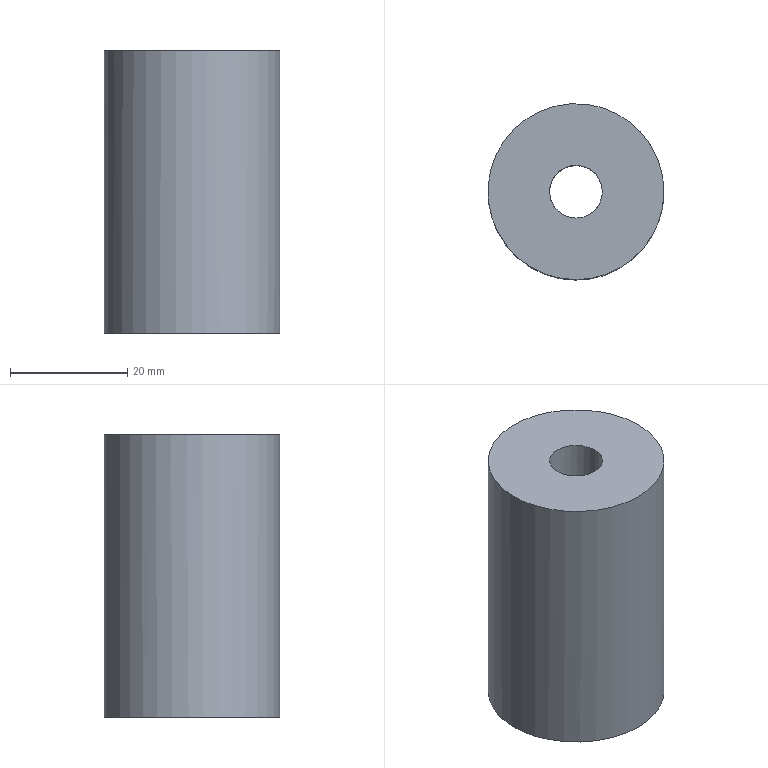Part | NX | features solid 2 | 1 solid | 6 faces | box 30 x 30 x 48.131 mm | volume 29431 mm3 | plane 3 | cylinder 3 | commonest cylinder face diameters 9.007 x1 14.508 x1 30 x1
STEP:
#1=CARTESIAN_POINT('',(1781.477,174.595,-113.132));
#2=VERTEX_POINT('',#1);
#3=CARTESIAN_POINT('',(1784.527,174.804,-113.132));
#4=CARTESIAN_POINT('',(1781.578,174.499,-113.132));
#5=CARTESIAN_POINT('',(1778.633,174.774,-113.132));
#6=CARTESIAN_POINT('',(1775.842,175.59,-113.132));
#7=CARTESIAN_POINT('',(1773.22,176.957,-113.132));
#8=CARTESIAN_POINT('',(1770.914,178.81,-113.132));
#9=CARTESIAN_POINT('',(1769.012,181.078,-113.132));
#10=CARTESIAN_POINT('',(1767.59,183.674,-113.132));
#11=CARTESIAN_POINT('',(1766.702,186.497,-113.132));
#12=CARTESIAN_POINT('',(1766.381,189.439,-113.132));
#13=CARTESIAN_POINT('',(1766.641,192.387,-113.132));
#14=CARTESIAN_POINT('',(1767.471,195.228,-113.132));
#15=CARTESIAN_POINT('',(1768.839,197.852,-113.132));
#16=CARTESIAN_POINT('',(1770.692,200.159,-113.132));
#17=CARTESIAN_POINT('',(1772.96,202.06,-113.132));
#18=CARTESIAN_POINT('',(1775.556,203.482,-113.132));
#19=CARTESIAN_POINT('',(1778.379,204.371,-113.132));
#20=CARTESIAN_POINT('',(1781.321,204.691,-113.132));
#21=CARTESIAN_POINT('',(1784.269,204.432,-113.132));
#22=CARTESIAN_POINT('',(1787.11,203.602,-113.132));
#23=CARTESIAN_POINT('',(1789.734,202.234,-113.132));
#24=CARTESIAN_POINT('',(1792.041,200.38,-113.132));
#25=CARTESIAN_POINT('',(1793.942,198.112,-113.132));
#26=CARTESIAN_POINT('',(1795.364,195.517,-113.132));
#27=CARTESIAN_POINT('',(1796.253,192.694,-113.132));
#28=CARTESIAN_POINT('',(1796.573,189.752,-113.132));
#29=CARTESIAN_POINT('',(1796.314,186.804,-113.132));
#30=CARTESIAN_POINT('',(1795.484,183.963,-113.132));
#31=CARTESIAN_POINT('',(1794.116,181.339,-113.132));
#32=CARTESIAN_POINT('',(1792.262,179.032,-113.132));
#33=CARTESIAN_POINT('',(1789.994,177.13,-113.132));
#34=CARTESIAN_POINT('',(1787.399,175.708,-113.132));
#35=CARTESIAN_POINT('',(1784.527,174.804,-113.132));
#36=CARTESIAN_POINT('',(1781.578,174.499,-113.132));
#37=CARTESIAN_POINT('',(1778.633,174.774,-113.132));
#38=B_SPLINE_CURVE_WITH_KNOTS('',3,(#3,#4,#5,#6,#7,#8,#9,#10,#11,#12,#13,#14,#15,#16,#17,#18,#19,#20,#21,#22,#23,#24,#25,#26,#27,#28,#29,#30,#31,#32,#33,#34,#35,#36,#37),.UNSPECIFIED.,.T.,.F.,(1,1,1,1,1,1,1,1,1,1,1,1,1,1,1,1,1,1,1,1,1,1,1,1,1,1,1,1,1,1,1,1,1,1,1,1,1,1,1),(-0.09539,-0.06414,-0.03289,0.,0.02969,0.06086,0.09211,0.1234,0.1546,0.1859,0.2171,0.2484,0.2796,0.3109,0.3421,0.3734,0.4046,0.4359,0.4671,0.4984,0.5296,0.5609,0.5921,0.6234,0.6546,0.6859,0.7171,0.7484,0.7796,0.8109,0.8421,0.8734,0.9046,0.9359,0.9671,1.,1.03,1.061,1.092),.UNSPECIFIED.);
#39=EDGE_CURVE('',#2,#2,#38,.F.);
#40=ORIENTED_EDGE('',*,*,#39,.F.);
#41=EDGE_LOOP('',(#40));
#42=FACE_BOUND('',#41,.T.);
#43=CARTESIAN_POINT('',(1779.999,182.493,-113.132));
#44=VERTEX_POINT('',#43);
#45=CARTESIAN_POINT('',(1781.477,189.595,-113.132));
#46=DIRECTION('',(-0.000000328,0.000000403,-1.));
#47=DIRECTION('',(-0.2037,-0.979,-0.000000328));
#48=AXIS2_PLACEMENT_3D('',#45,#46,#47);
#49=CIRCLE('',#48,7.254);
#50=EDGE_CURVE('',#44,#44,#49,.F.);
#51=ORIENTED_EDGE('',*,*,#50,.T.);
#52=EDGE_LOOP('',(#51));
#53=FACE_BOUND('',#52,.T.);
#54=CARTESIAN_POINT('',(1785.543,185.529,-113.132));
#55=DIRECTION('',(0.000000328,-0.000000403,1.));
#56=DIRECTION('',(-0.7071,-0.7071,-0.000000053));
#57=AXIS2_PLACEMENT_3D('',#54,#55,#56);
#58=PLANE('',#57);
#59=ADVANCED_FACE('',(#42,#53),#58,.F.);
#60=CARTESIAN_POINT('',(1796.477,189.595,-65.001));
#61=VERTEX_POINT('',#60);
#62=CARTESIAN_POINT('',(1781.477,189.595,-65.001));
#63=DIRECTION('',(0.,0.,-1.));
#64=DIRECTION('',(1.,0.,0.));
#65=AXIS2_PLACEMENT_3D('',#62,#63,#64);
#66=CIRCLE('',#65,15.);
#67=EDGE_CURVE('',#61,#61,#66,.T.);
#68=ORIENTED_EDGE('',*,*,#67,.T.);
#69=EDGE_LOOP('',(#68));
#70=FACE_BOUND('',#69,.T.);
#71=ORIENTED_EDGE('',*,*,#39,.T.);
#72=EDGE_LOOP('',(#71));
#73=FACE_BOUND('',#72,.T.);
#74=CARTESIAN_POINT('',(1781.477,189.595,-119.132));
#75=DIRECTION('',(0.000000328,-0.000000403,1.));
#76=DIRECTION('',(-0.2037,-0.979,-0.000000328));
#77=AXIS2_PLACEMENT_3D('',#74,#75,#76);
#78=CYLINDRICAL_SURFACE('',#77,15.);
#79=ADVANCED_FACE('',(#70,#73),#78,.T.);
#80=CARTESIAN_POINT('',(1785.981,189.595,-65.001));
#81=VERTEX_POINT('',#80);
#82=CARTESIAN_POINT('',(1781.477,189.595,-65.001));
#83=DIRECTION('',(0.,0.,-1.));
#84=DIRECTION('',(1.,0.,0.));
#85=AXIS2_PLACEMENT_3D('',#82,#83,#84);
#86=CIRCLE('',#85,4.503);
#87=EDGE_CURVE('',#81,#81,#86,.F.);
#88=ORIENTED_EDGE('',*,*,#87,.T.);
#89=EDGE_LOOP('',(#88));
#90=FACE_BOUND('',#89,.T.);
#91=CARTESIAN_POINT('',(1781.477,185.092,-98.132));
#92=VERTEX_POINT('',#91);
#93=CARTESIAN_POINT('',(1780.562,185.155,-98.132));
#94=CARTESIAN_POINT('',(1781.447,185.063,-98.132));
#95=CARTESIAN_POINT('',(1782.331,185.145,-98.132));
#96=CARTESIAN_POINT('',(1783.169,185.39,-98.132));
#97=CARTESIAN_POINT('',(1783.956,185.801,-98.132));
#98=CARTESIAN_POINT('',(1784.649,186.357,-98.132));
#99=CARTESIAN_POINT('',(1785.22,187.038,-98.132));
#100=CARTESIAN_POINT('',(1785.647,187.817,-98.132));
#101=CARTESIAN_POINT('',(1785.913,188.665,-98.132));
#102=CARTESIAN_POINT('',(1786.01,189.548,-98.132));
#103=CARTESIAN_POINT('',(1785.932,190.433,-98.132));
#104=CARTESIAN_POINT('',(1785.683,191.286,-98.132));
#105=CARTESIAN_POINT('',(1785.272,192.074,-98.132));
#106=CARTESIAN_POINT('',(1784.715,192.767,-98.132));
#107=CARTESIAN_POINT('',(1784.034,193.338,-98.132));
#108=CARTESIAN_POINT('',(1783.255,193.765,-98.132));
#109=CARTESIAN_POINT('',(1782.408,194.031,-98.132));
#110=CARTESIAN_POINT('',(1781.524,194.128,-98.132));
#111=CARTESIAN_POINT('',(1780.639,194.05,-98.132));
#112=CARTESIAN_POINT('',(1779.786,193.801,-98.132));
#113=CARTESIAN_POINT('',(1778.998,193.39,-98.132));
#114=CARTESIAN_POINT('',(1778.306,192.833,-98.132));
#115=CARTESIAN_POINT('',(1777.735,192.152,-98.132));
#116=CARTESIAN_POINT('',(1777.308,191.373,-98.132));
#117=CARTESIAN_POINT('',(1777.041,190.526,-98.132));
#118=CARTESIAN_POINT('',(1776.945,189.642,-98.132));
#119=CARTESIAN_POINT('',(1777.023,188.757,-98.132));
#120=CARTESIAN_POINT('',(1777.272,187.904,-98.132));
#121=CARTESIAN_POINT('',(1777.683,187.116,-98.132));
#122=CARTESIAN_POINT('',(1778.239,186.424,-98.132));
#123=CARTESIAN_POINT('',(1778.92,185.853,-98.132));
#124=CARTESIAN_POINT('',(1779.699,185.426,-98.132));
#125=CARTESIAN_POINT('',(1780.562,185.155,-98.132));
#126=CARTESIAN_POINT('',(1781.447,185.063,-98.132));
#127=CARTESIAN_POINT('',(1782.331,185.145,-98.132));
#128=B_SPLINE_CURVE_WITH_KNOTS('',3,(#93,#94,#95,#96,#97,#98,#99,#100,#101,#102,#103,#104,#105,#106,#107,#108,#109,#110,#111,#112,#113,#114,#115,#116,#117,#118,#119,#120,#121,#122,#123,#124,#125,#126,#127),.UNSPECIFIED.,.T.,.F.,(1,1,1,1,1,1,1,1,1,1,1,1,1,1,1,1,1,1,1,1,1,1,1,1,1,1,1,1,1,1,1,1,1,1,1,1,1,1,1),(-0.09539,-0.06414,-0.03289,0.,0.02969,0.06086,0.09211,0.1234,0.1546,0.1859,0.2171,0.2484,0.2796,0.3109,0.3421,0.3734,0.4046,0.4359,0.4671,0.4984,0.5296,0.5609,0.5921,0.6234,0.6546,0.6859,0.7171,0.7484,0.7796,0.8109,0.8421,0.8734,0.9046,0.9359,0.9671,1.,1.03,1.061,1.092),.UNSPECIFIED.);
#129=EDGE_CURVE('',#92,#92,#128,.T.);
#130=ORIENTED_EDGE('',*,*,#129,.F.);
#131=EDGE_LOOP('',(#130));
#132=FACE_BOUND('',#131,.T.);
#133=CARTESIAN_POINT('',(1781.477,189.595,-111.132));
#134=DIRECTION('',(0.000000328,-0.000000403,1.));
#135=DIRECTION('',(-0.2037,-0.979,-0.000000328));
#136=AXIS2_PLACEMENT_3D('',#133,#134,#135);
#137=CYLINDRICAL_SURFACE('',#136,4.503);
#138=ADVANCED_FACE('',(#90,#132),#137,.F.);
#139=ORIENTED_EDGE('',*,*,#129,.T.);
#140=EDGE_LOOP('',(#139));
#141=FACE_BOUND('',#140,.T.);
#142=CARTESIAN_POINT('',(1779.999,182.493,-98.132));
#143=VERTEX_POINT('',#142);
#144=CARTESIAN_POINT('',(1781.477,189.595,-98.132));
#145=DIRECTION('',(0.000000328,-0.000000403,1.));
#146=DIRECTION('',(-0.2037,-0.979,-0.000000328));
#147=AXIS2_PLACEMENT_3D('',#144,#145,#146);
#148=CIRCLE('',#147,7.254);
#149=EDGE_CURVE('',#143,#143,#148,.T.);
#150=ORIENTED_EDGE('',*,*,#149,.F.);
#151=EDGE_LOOP('',(#150));
#152=FACE_BOUND('',#151,.T.);
#153=CARTESIAN_POINT('',(1781.477,189.595,-98.132));
#154=DIRECTION('',(0.000000328,-0.000000403,1.));
#155=DIRECTION('',(0.,-1.,-0.000000403));
#156=AXIS2_PLACEMENT_3D('',#153,#154,#155);
#157=PLANE('',#156);
#158=ADVANCED_FACE('',(#141,#152),#157,.F.);
#159=ORIENTED_EDGE('',*,*,#149,.T.);
#160=EDGE_LOOP('',(#159));
#161=FACE_BOUND('',#160,.T.);
#162=ORIENTED_EDGE('',*,*,#50,.F.);
#163=EDGE_LOOP('',(#162));
#164=FACE_BOUND('',#163,.T.);
#165=CARTESIAN_POINT('',(1781.477,189.595,-113.132));
#166=DIRECTION('',(0.000000328,-0.000000403,1.));
#167=DIRECTION('',(-0.2037,-0.979,-0.000000328));
#168=AXIS2_PLACEMENT_3D('',#165,#166,#167);
#169=CYLINDRICAL_SURFACE('',#168,7.254);
#170=ADVANCED_FACE('',(#161,#164),#169,.F.);
#171=ORIENTED_EDGE('',*,*,#67,.F.);
#172=EDGE_LOOP('',(#171));
#173=FACE_BOUND('',#172,.T.);
#174=ORIENTED_EDGE('',*,*,#87,.F.);
#175=EDGE_LOOP('',(#174));
#176=FACE_BOUND('',#175,.T.);
#177=CARTESIAN_POINT('',(1770.977,112.546,-65.001));
#178=DIRECTION('',(0.,0.,-1.));
#179=DIRECTION('',(1.,0.,0.));
#180=AXIS2_PLACEMENT_3D('',#177,#178,#179);
#181=PLANE('',#180);
#182=ADVANCED_FACE('',(#173,#176),#181,.F.);
#183=CLOSED_SHELL('',(#59,#79,#138,#158,#170,#182));
#184=MANIFOLD_SOLID_BREP('',#183);
#185=(LENGTH_UNIT()NAMED_UNIT(*)SI_UNIT(.MILLI.,.METRE.));
#186=UNCERTAINTY_MEASURE_WITH_UNIT(LENGTH_MEASURE(0.0508),#185,'','');
#187=(NAMED_UNIT(*)PLANE_ANGLE_UNIT()SI_UNIT($,.RADIAN.));
#188=(NAMED_UNIT(*)SI_UNIT($,.STERADIAN.)SOLID_ANGLE_UNIT());
#189=(GEOMETRIC_REPRESENTATION_CONTEXT(3)GLOBAL_UNCERTAINTY_ASSIGNED_CONTEXT((#186))GLOBAL_UNIT_ASSIGNED_CONTEXT((#185,#187,#188))REPRESENTATION_CONTEXT('',''));
#190=ADVANCED_BREP_SHAPE_REPRESENTATION('',(#184),#189);